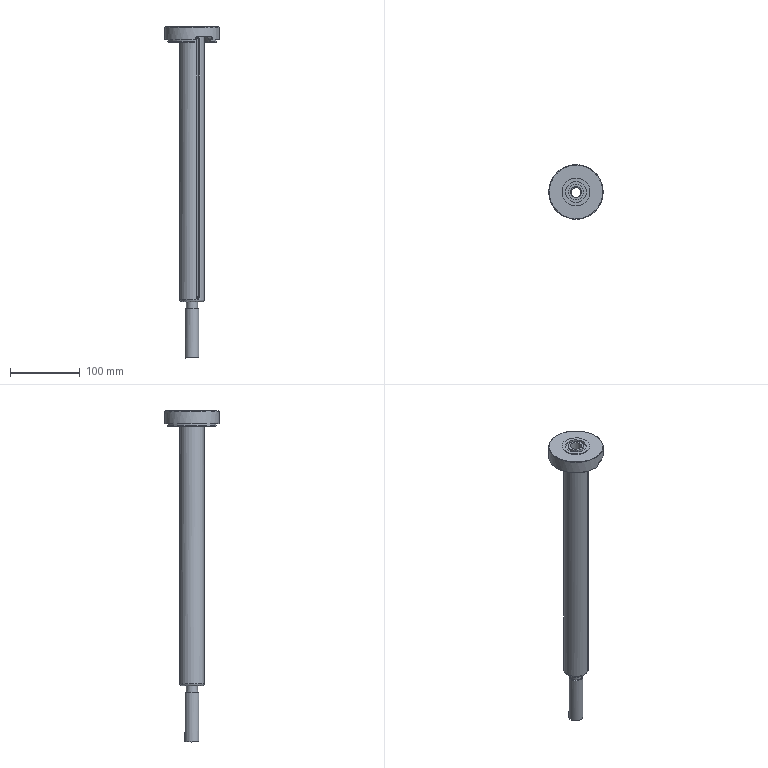Part | STEP file | solid 198 | 1 solid | 51 faces | box 78 x 78 x 475.57 mm | volume 368550 mm3 | plane 21 | cylinder 15 | spline 7 | cone 5 | sphere 2 | torus 1 | commonest cylinder face diameters 5 x3 10 x2 16 x2 14 x1 20 x1 22 x1